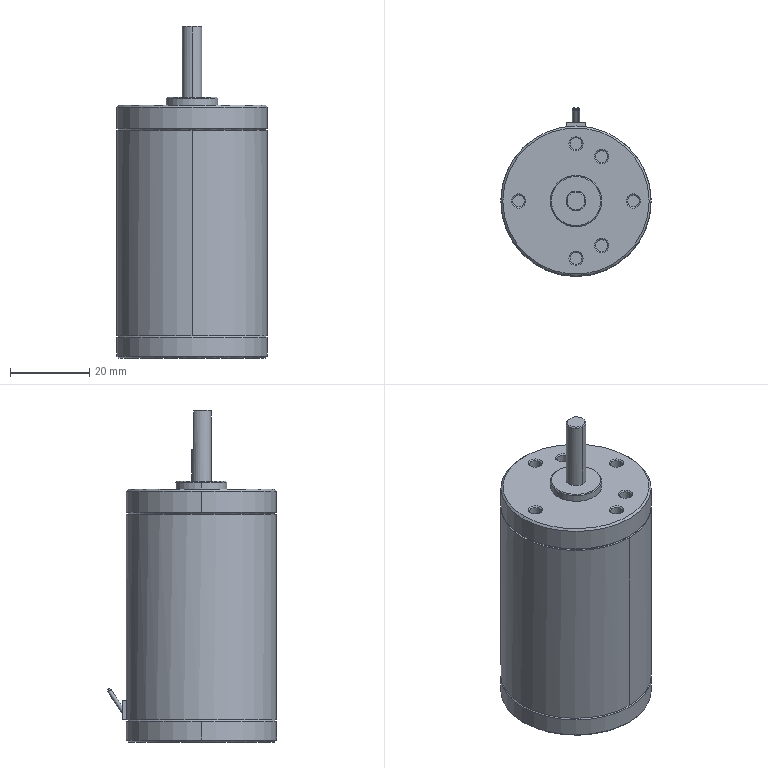Part | SolidWorks | features Chamfer 4, Revolution 4, ICE 3, MirrorPattern 1, RefAxis 1 | 3 solids | 71 faces | box 38 x 42.771 x 84 mm | volume 72893 mm3 | cylinder 30 | cone 23 | plane 18 | commonest cylinder face diameters 3 x12 38 x6 0.5 x4 1 x4 5 x2 13 x2